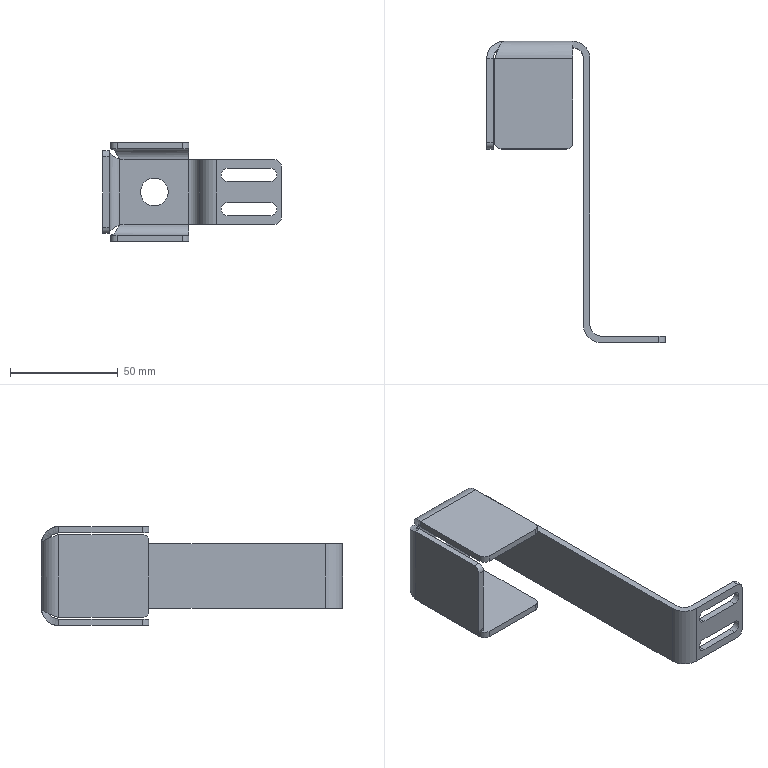Part | NX | features BREP 1 | 1 solid | 55 faces | box 83 x 140 x 46 mm | volume 34393 mm3 | plane 28 | cylinder 23 | spline 4 | commonest cylinder face diameters 6 x12 10 x5 16 x5 13 x1